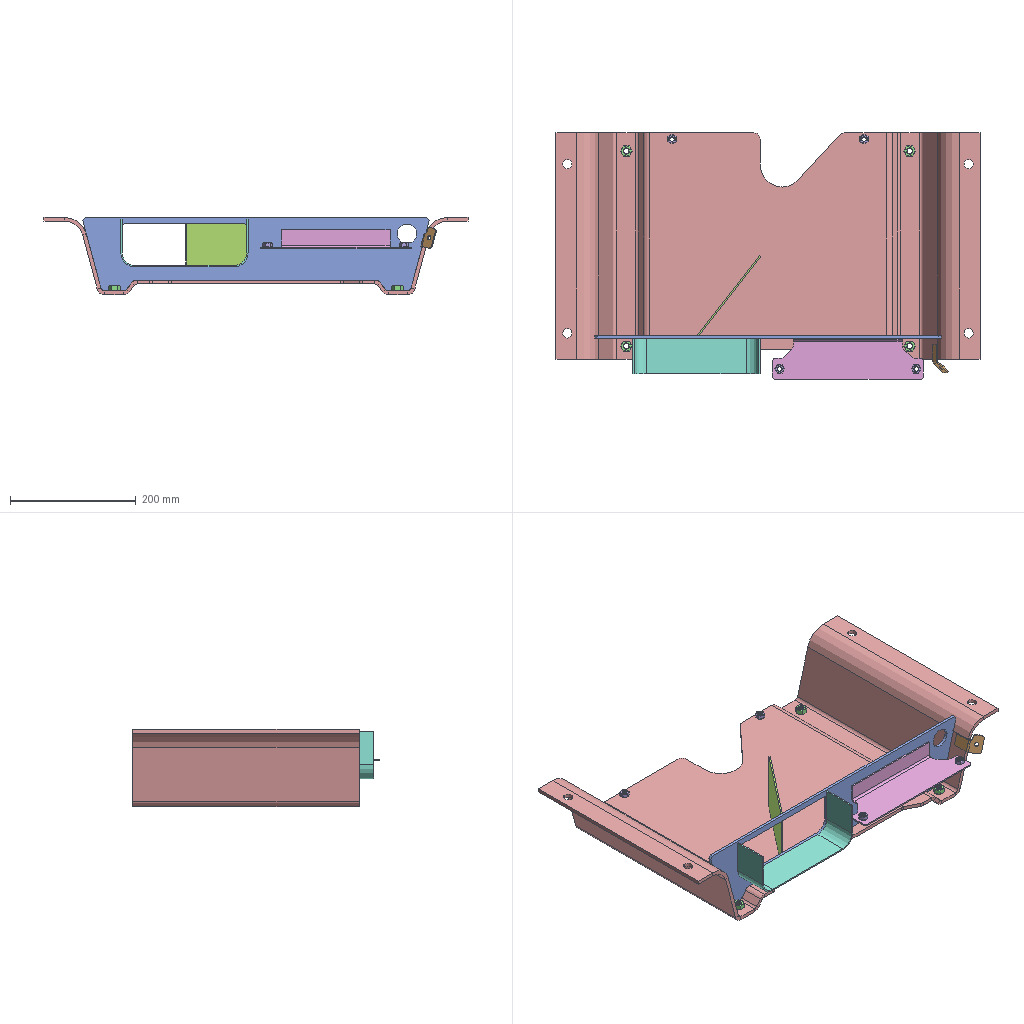Assembly | SolidWorks | 7 different items | 14 placed | box 674 x 392 x 123 mm
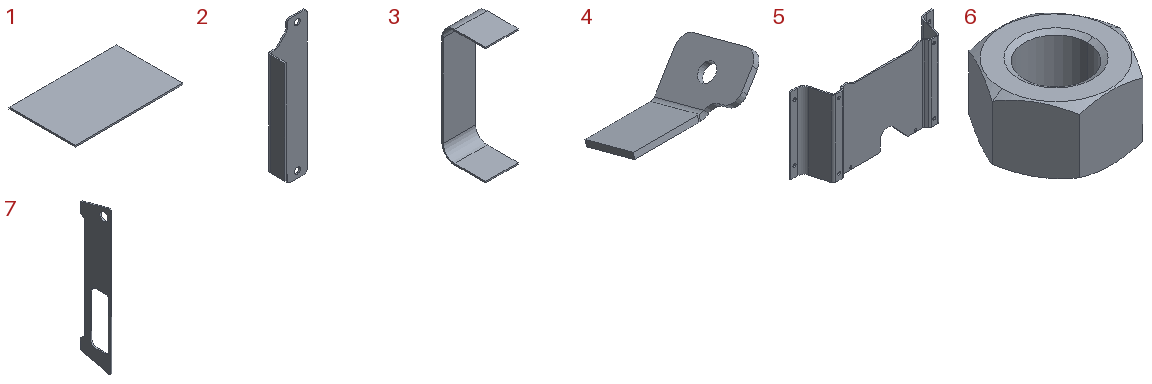Parts list (item | quantity | size | volume | features):
1 | x1 | 160 x 97.8 x 2.3 mm | 35990 mm3 | features FlatPattern 1, SMBaseFlange 1, SheetMetal 1
2 | x1 | 65 x 30 x 240 mm | 41523 mm3 | features BaseBody 1, FlatPattern 1, SheetMetal 1, SolidToSheetMetal 1
3 | x1 | 56 x 75.7 x 202.6 mm | 42664 mm3 | features BaseBody 1, FlatPattern 1, SheetMetal 1, SolidToSheetMetal 1
4 | x1 | 44.304 x 32.939 x 24.3 mm | 2673 mm3 | features BaseBody 1, FlatPattern 1, SheetMetal 1, SolidToSheetMetal 1
5 | x1 | 674 x 122.8 x 360 mm | 1751347 mm3 | features Fillet 2, ICE 2, FlatPattern 1, SMBaseFlange 1, SheetMetal 1
6 | x8 | 34.641 x 30 x 18 mm | 9644 mm3 | features RevCut 2, Chamfer 1, Extrusion 1, LPattern 1
7 | x1 | 4.5 x 116.8 x 550.797 mm | 181763 mm3 | features BaseBody 1
Mates (type | each side: item.copy, entity, surface, feature):
Coincident | 5.1 face plane Base-Flange1 | 7.1 face plane Input1 | 2 times
DistanceDim | 7.1 face plane Input1 | 5.1 face plane Base-Flange1
Coincident | 5.1 face plane Base-Flange1 | 1.1 face plane Base-Flange1
PlanarAngleDim | 1.1 face plane Base-Flange1 | 7.1 face plane Input1
Coincident | 7.1 face plane Input1 | 1.1 edge
DistanceDim | 7.1 face plane Input1 | 1.1 edge
Concentric | 5.1 face cylinder Cut-Extrude1 | 6.1 face cone EndChamfer
Coincident | 5.1 face plane Base-Flange1 | 6.1 face plane BaseNut
Concentric | 5.1 face cylinder Cut-Extrude1 | 6.2 face cone EndChamfer
Coincident | 5.1 face plane Base-Flange1 | 6.2 face plane BaseNut
Concentric | 5.1 face cylinder Cut-Extrude1 | 6.3 face cone EndChamfer
Coincident | 5.1 face plane Base-Flange1 | 6.3 face plane BaseNut
Concentric | 5.1 face cylinder Cut-Extrude1 | 6.4 face cone EndChamfer
Coincident | 5.1 face plane Base-Flange1 | 6.4 face plane BaseNut
Concentric | 5.1 face cylinder Cut-Extrude1 | 6.5 face cone EndChamfer
Coincident | 5.1 face plane Base-Flange1 | 6.5 face plane BaseNut
Concentric | 5.1 face cylinder Cut-Extrude1 | 6.6 face cone EndChamfer
Coincident | 5.1 face plane Base-Flange1 | 6.6 face plane BaseNut
Parallel | 5.1 face plane Base-Flange1 | 6.5 face plane BaseNut
Parallel | 5.1 face plane Base-Flange1 | 6.6 face plane BaseNut